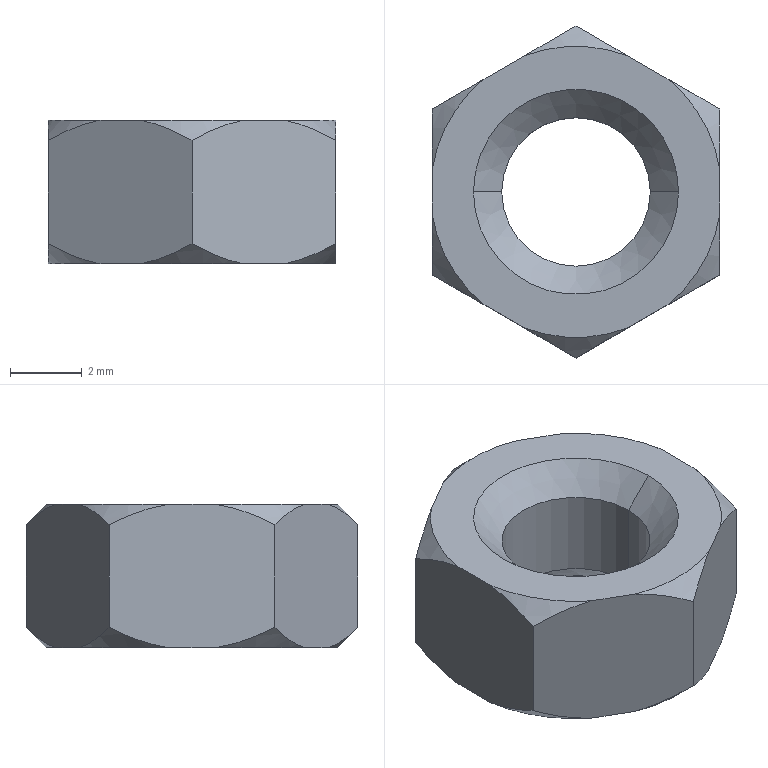Part | NX | features BREP 1 | 1 solid | 26 faces | box 8 x 9.238 x 4 mm | volume 157.518 mm3 | cone 16 | plane 8 | cylinder 2 | commonest cylinder face diameters 4.134 x2
STEP:
#1=CARTESIAN_POINT('',(-2.067,0.,-3.213));
#2=VERTEX_POINT('',#1);
#3=CARTESIAN_POINT('',(2.067,0.,-3.213));
#4=VERTEX_POINT('',#3);
#5=CARTESIAN_POINT('',(0.,0.,-3.213));
#6=DIRECTION('',(0.,0.,1.));
#7=DIRECTION('',(1.,0.,0.));
#8=AXIS2_PLACEMENT_3D('',#5,#6,#7);
#9=CIRCLE('',#8,2.067);
#10=EDGE_CURVE('',#2,#4,#9,.T.);
#11=ORIENTED_EDGE('',*,*,#10,.T.);
#12=CARTESIAN_POINT('',(2.854,0.,-4.));
#13=VERTEX_POINT('',#12);
#14=CARTESIAN_POINT('',(2.067,0.,-3.213));
#15=DIRECTION('',(0.7071,0.,-0.7071));
#16=VECTOR('',#15,1000.);
#17=LINE('',#14,#16);
#18=EDGE_CURVE('',#13,#4,#17,.F.);
#19=ORIENTED_EDGE('',*,*,#18,.F.);
#20=CARTESIAN_POINT('',(-2.854,0.,-4.));
#21=VERTEX_POINT('',#20);
#22=CARTESIAN_POINT('',(0.,0.,-4.));
#23=DIRECTION('',(0.,0.,1.));
#24=DIRECTION('',(1.,0.,0.));
#25=AXIS2_PLACEMENT_3D('',#22,#23,#24);
#26=CIRCLE('',#25,2.854);
#27=EDGE_CURVE('',#21,#13,#26,.T.);
#28=ORIENTED_EDGE('',*,*,#27,.F.);
#29=CARTESIAN_POINT('',(-2.067,0.,-3.213));
#30=DIRECTION('',(-0.7071,0.,-0.7071));
#31=VECTOR('',#30,1000.);
#32=LINE('',#29,#31);
#33=EDGE_CURVE('',#21,#2,#32,.F.);
#34=ORIENTED_EDGE('',*,*,#33,.T.);
#35=EDGE_LOOP('',(#11,#19,#28,#34));
#36=FACE_BOUND('',#35,.T.);
#37=CARTESIAN_POINT('',(0.,0.,-3.213));
#38=DIRECTION('',(0.,0.,-1.));
#39=DIRECTION('',(1.,0.,0.));
#40=AXIS2_PLACEMENT_3D('',#37,#38,#39);
#41=CONICAL_SURFACE('',#40,2.067,0.7854);
#42=ADVANCED_FACE('',(#36),#41,.F.);
#43=ORIENTED_EDGE('',*,*,#10,.F.);
#44=CARTESIAN_POINT('',(-2.067,0.,-0.7866));
#45=VERTEX_POINT('',#44);
#46=CARTESIAN_POINT('',(-2.067,0.,-23.));
#47=DIRECTION('',(0.,0.,1.));
#48=VECTOR('',#47,1000.);
#49=LINE('',#46,#48);
#50=EDGE_CURVE('',#2,#45,#49,.T.);
#51=ORIENTED_EDGE('',*,*,#50,.T.);
#52=CARTESIAN_POINT('',(2.067,0.,-0.7866));
#53=VERTEX_POINT('',#52);
#54=CARTESIAN_POINT('',(0.,0.,-0.7866));
#55=DIRECTION('',(0.,0.,1.));
#56=DIRECTION('',(1.,0.,0.));
#57=AXIS2_PLACEMENT_3D('',#54,#55,#56);
#58=CIRCLE('',#57,2.067);
#59=EDGE_CURVE('',#45,#53,#58,.T.);
#60=ORIENTED_EDGE('',*,*,#59,.T.);
#61=CARTESIAN_POINT('',(2.067,0.,-23.));
#62=DIRECTION('',(0.,0.,1.));
#63=VECTOR('',#62,1000.);
#64=LINE('',#61,#63);
#65=EDGE_CURVE('',#4,#53,#64,.T.);
#66=ORIENTED_EDGE('',*,*,#65,.F.);
#67=EDGE_LOOP('',(#43,#51,#60,#66));
#68=FACE_BOUND('',#67,.T.);
#69=CARTESIAN_POINT('',(0.,0.,-23.));
#70=DIRECTION('',(0.,0.,1.));
#71=DIRECTION('',(-1.,0.,0.));
#72=AXIS2_PLACEMENT_3D('',#69,#70,#71);
#73=CYLINDRICAL_SURFACE('',#72,2.067);
#74=ADVANCED_FACE('',(#68),#73,.F.);
#75=ORIENTED_EDGE('',*,*,#59,.F.);
#76=CARTESIAN_POINT('',(-2.854,0.,0.));
#77=VERTEX_POINT('',#76);
#78=CARTESIAN_POINT('',(-2.854,0.,0.));
#79=DIRECTION('',(-0.7071,0.,0.7071));
#80=VECTOR('',#79,1000.);
#81=LINE('',#78,#80);
#82=EDGE_CURVE('',#45,#77,#81,.T.);
#83=ORIENTED_EDGE('',*,*,#82,.T.);
#84=CARTESIAN_POINT('',(2.854,0.,0.));
#85=VERTEX_POINT('',#84);
#86=CARTESIAN_POINT('',(0.,0.,0.));
#87=DIRECTION('',(0.,0.,1.));
#88=DIRECTION('',(1.,0.,0.));
#89=AXIS2_PLACEMENT_3D('',#86,#87,#88);
#90=CIRCLE('',#89,2.854);
#91=EDGE_CURVE('',#77,#85,#90,.T.);
#92=ORIENTED_EDGE('',*,*,#91,.T.);
#93=CARTESIAN_POINT('',(2.854,0.,0.));
#94=DIRECTION('',(0.7071,0.,0.7071));
#95=VECTOR('',#94,1000.);
#96=LINE('',#93,#95);
#97=EDGE_CURVE('',#53,#85,#96,.T.);
#98=ORIENTED_EDGE('',*,*,#97,.F.);
#99=EDGE_LOOP('',(#75,#83,#92,#98));
#100=FACE_BOUND('',#99,.T.);
#101=CARTESIAN_POINT('',(0.,0.,0.));
#102=DIRECTION('',(0.,0.,1.));
#103=DIRECTION('',(-1.,0.,0.));
#104=AXIS2_PLACEMENT_3D('',#101,#102,#103);
#105=CONICAL_SURFACE('',#104,2.854,0.7854);
#106=ADVANCED_FACE('',(#100),#105,.F.);
#107=CARTESIAN_POINT('',(-4.,0.6483,0.));
#108=VERTEX_POINT('',#107);
#109=CARTESIAN_POINT('',(-4.,2.309,-0.5666));
#110=VERTEX_POINT('',#109);
#111=CARTESIAN_POINT('',(-4.,0.6483,0.));
#112=CARTESIAN_POINT('',(-4.,1.234,-0.09377));
#113=CARTESIAN_POINT('',(-4.,1.781,-0.3026));
#114=CARTESIAN_POINT('',(-4.,2.309,-0.5666));
#115=B_SPLINE_CURVE_WITH_KNOTS('',3,(#111,#112,#113,#114),.UNSPECIFIED.,.F.,.F.,(4,4),(0.,0.001755),.UNSPECIFIED.);
#116=EDGE_CURVE('',#108,#110,#115,.T.);
#117=ORIENTED_EDGE('',*,*,#116,.F.);
#118=CARTESIAN_POINT('',(-2.561,3.14,0.));
#119=VERTEX_POINT('',#118);
#120=CARTESIAN_POINT('',(0.,0.,0.));
#121=DIRECTION('',(0.,0.,1.));
#122=DIRECTION('',(1.,0.,0.));
#123=AXIS2_PLACEMENT_3D('',#120,#121,#122);
#124=CIRCLE('',#123,4.052);
#125=EDGE_CURVE('',#119,#108,#124,.T.);
#126=ORIENTED_EDGE('',*,*,#125,.F.);
#127=CARTESIAN_POINT('',(-4.,2.309,-0.5666));
#128=CARTESIAN_POINT('',(-3.543,2.573,-0.3026));
#129=CARTESIAN_POINT('',(-3.069,2.847,-0.09377));
#130=CARTESIAN_POINT('',(-2.561,3.14,0.));
#131=B_SPLINE_CURVE_WITH_KNOTS('',3,(#127,#128,#129,#130),.UNSPECIFIED.,.F.,.F.,(4,4),(0.,0.001755),.UNSPECIFIED.);
#132=EDGE_CURVE('',#110,#119,#131,.T.);
#133=ORIENTED_EDGE('',*,*,#132,.F.);
#134=EDGE_LOOP('',(#117,#126,#133));
#135=FACE_BOUND('',#134,.T.);
#136=CARTESIAN_POINT('',(0.,0.,-0.9428));
#137=DIRECTION('',(0.,0.,-1.));
#138=DIRECTION('',(1.,0.,0.));
#139=AXIS2_PLACEMENT_3D('',#136,#137,#138);
#140=CONICAL_SURFACE('',#139,4.995,0.7854);
#141=ADVANCED_FACE('',(#135),#140,.T.);
#142=CARTESIAN_POINT('',(-1.439,3.788,0.));
#143=VERTEX_POINT('',#142);
#144=CARTESIAN_POINT('',(0.,4.619,-0.5666));
#145=VERTEX_POINT('',#144);
#146=CARTESIAN_POINT('',(-1.439,3.788,0.));
#147=CARTESIAN_POINT('',(-1.187,3.933,-0.04639));
#148=CARTESIAN_POINT('',(-0.9421,4.075,-0.122));
#149=CARTESIAN_POINT('',(-0.4604,4.353,-0.3173));
#150=CARTESIAN_POINT('',(-0.2261,4.488,-0.4361));
#151=CARTESIAN_POINT('',(0.,4.619,-0.5666));
#152=B_SPLINE_CURVE_WITH_KNOTS('',3,(#146,#147,#148,#149,#150,#151),.UNSPECIFIED.,.F.,.F.,(4,2,4),(0.,0.5,1.),.UNSPECIFIED.);
#153=EDGE_CURVE('',#143,#145,#152,.T.);
#154=ORIENTED_EDGE('',*,*,#153,.F.);
#155=CARTESIAN_POINT('',(1.439,3.788,0.));
#156=VERTEX_POINT('',#155);
#157=CARTESIAN_POINT('',(0.,0.,0.));
#158=DIRECTION('',(0.,0.,1.));
#159=DIRECTION('',(1.,0.,0.));
#160=AXIS2_PLACEMENT_3D('',#157,#158,#159);
#161=CIRCLE('',#160,4.052);
#162=EDGE_CURVE('',#156,#143,#161,.T.);
#163=ORIENTED_EDGE('',*,*,#162,.F.);
#164=CARTESIAN_POINT('',(0.,4.619,-0.5666));
#165=CARTESIAN_POINT('',(0.4573,4.355,-0.3026));
#166=CARTESIAN_POINT('',(0.931,4.081,-0.09377));
#167=CARTESIAN_POINT('',(1.439,3.788,0.));
#168=B_SPLINE_CURVE_WITH_KNOTS('',3,(#164,#165,#166,#167),.UNSPECIFIED.,.F.,.F.,(4,4),(0.,0.001755),.UNSPECIFIED.);
#169=EDGE_CURVE('',#145,#156,#168,.T.);
#170=ORIENTED_EDGE('',*,*,#169,.F.);
#171=EDGE_LOOP('',(#154,#163,#170));
#172=FACE_BOUND('',#171,.T.);
#173=CARTESIAN_POINT('',(0.,0.,-0.9428));
#174=DIRECTION('',(0.,0.,-1.));
#175=DIRECTION('',(1.,0.,0.));
#176=AXIS2_PLACEMENT_3D('',#173,#174,#175);
#177=CONICAL_SURFACE('',#176,4.995,0.7854);
#178=ADVANCED_FACE('',(#172),#177,.T.);
#179=CARTESIAN_POINT('',(2.561,3.14,0.));
#180=VERTEX_POINT('',#179);
#181=CARTESIAN_POINT('',(4.,2.309,-0.5666));
#182=VERTEX_POINT('',#181);
#183=CARTESIAN_POINT('',(2.561,3.14,0.));
#184=CARTESIAN_POINT('',(2.813,2.995,-0.04639));
#185=CARTESIAN_POINT('',(3.058,2.853,-0.122));
#186=CARTESIAN_POINT('',(3.54,2.575,-0.3173));
#187=CARTESIAN_POINT('',(3.774,2.44,-0.4361));
#188=CARTESIAN_POINT('',(4.,2.309,-0.5666));
#189=B_SPLINE_CURVE_WITH_KNOTS('',3,(#183,#184,#185,#186,#187,#188),.UNSPECIFIED.,.F.,.F.,(4,2,4),(0.,0.5,1.),.UNSPECIFIED.);
#190=EDGE_CURVE('',#180,#182,#189,.T.);
#191=ORIENTED_EDGE('',*,*,#190,.F.);
#192=CARTESIAN_POINT('',(4.,0.6483,0.));
#193=VERTEX_POINT('',#192);
#194=CARTESIAN_POINT('',(0.,0.,0.));
#195=DIRECTION('',(0.,0.,1.));
#196=DIRECTION('',(1.,0.,0.));
#197=AXIS2_PLACEMENT_3D('',#194,#195,#196);
#198=CIRCLE('',#197,4.052);
#199=EDGE_CURVE('',#193,#180,#198,.T.);
#200=ORIENTED_EDGE('',*,*,#199,.F.);
#201=CARTESIAN_POINT('',(4.,2.309,-0.5666));
#202=CARTESIAN_POINT('',(4.,1.781,-0.3026));
#203=CARTESIAN_POINT('',(4.,1.234,-0.09377));
#204=CARTESIAN_POINT('',(4.,0.6483,0.));
#205=B_SPLINE_CURVE_WITH_KNOTS('',3,(#201,#202,#203,#204),.UNSPECIFIED.,.F.,.F.,(4,4),(0.,0.001755),.UNSPECIFIED.);
#206=EDGE_CURVE('',#182,#193,#205,.T.);
#207=ORIENTED_EDGE('',*,*,#206,.F.);
#208=EDGE_LOOP('',(#191,#200,#207));
#209=FACE_BOUND('',#208,.T.);
#210=CARTESIAN_POINT('',(0.,0.,-0.9428));
#211=DIRECTION('',(0.,0.,-1.));
#212=DIRECTION('',(1.,0.,0.));
#213=AXIS2_PLACEMENT_3D('',#210,#211,#212);
#214=CONICAL_SURFACE('',#213,4.995,0.7854);
#215=ADVANCED_FACE('',(#209),#214,.T.);
#216=CARTESIAN_POINT('',(4.,-0.6483,0.));
#217=VERTEX_POINT('',#216);
#218=CARTESIAN_POINT('',(4.,-2.309,-0.5666));
#219=VERTEX_POINT('',#218);
#220=CARTESIAN_POINT('',(4.,-0.6483,0.));
#221=CARTESIAN_POINT('',(4.,-1.234,-0.09377));
#222=CARTESIAN_POINT('',(4.,-1.781,-0.3026));
#223=CARTESIAN_POINT('',(4.,-2.309,-0.5666));
#224=B_SPLINE_CURVE_WITH_KNOTS('',3,(#220,#221,#222,#223),.UNSPECIFIED.,.F.,.F.,(4,4),(0.,0.001755),.UNSPECIFIED.);
#225=EDGE_CURVE('',#217,#219,#224,.T.);
#226=ORIENTED_EDGE('',*,*,#225,.F.);
#227=CARTESIAN_POINT('',(2.561,-3.14,0.));
#228=VERTEX_POINT('',#227);
#229=CARTESIAN_POINT('',(0.,0.,0.));
#230=DIRECTION('',(0.,0.,1.));
#231=DIRECTION('',(1.,0.,0.));
#232=AXIS2_PLACEMENT_3D('',#229,#230,#231);
#233=CIRCLE('',#232,4.052);
#234=EDGE_CURVE('',#228,#217,#233,.T.);
#235=ORIENTED_EDGE('',*,*,#234,.F.);
#236=CARTESIAN_POINT('',(4.,-2.309,-0.5666));
#237=CARTESIAN_POINT('',(3.543,-2.573,-0.3026));
#238=CARTESIAN_POINT('',(3.069,-2.847,-0.09377));
#239=CARTESIAN_POINT('',(2.561,-3.14,0.));
#240=B_SPLINE_CURVE_WITH_KNOTS('',3,(#236,#237,#238,#239),.UNSPECIFIED.,.F.,.F.,(4,4),(0.,0.001755),.UNSPECIFIED.);
#241=EDGE_CURVE('',#219,#228,#240,.T.);
#242=ORIENTED_EDGE('',*,*,#241,.F.);
#243=EDGE_LOOP('',(#226,#235,#242));
#244=FACE_BOUND('',#243,.T.);
#245=CARTESIAN_POINT('',(0.,0.,-0.9428));
#246=DIRECTION('',(0.,0.,-1.));
#247=DIRECTION('',(1.,0.,0.));
#248=AXIS2_PLACEMENT_3D('',#245,#246,#247);
#249=CONICAL_SURFACE('',#248,4.995,0.7854);
#250=ADVANCED_FACE('',(#244),#249,.T.);
#251=CARTESIAN_POINT('',(1.439,-3.788,0.));
#252=VERTEX_POINT('',#251);
#253=CARTESIAN_POINT('',(0.,-4.619,-0.5666));
#254=VERTEX_POINT('',#253);
#255=CARTESIAN_POINT('',(1.439,-3.788,0.));
#256=CARTESIAN_POINT('',(1.187,-3.933,-0.04639));
#257=CARTESIAN_POINT('',(0.9421,-4.075,-0.122));
#258=CARTESIAN_POINT('',(0.4604,-4.353,-0.3173));
#259=CARTESIAN_POINT('',(0.2261,-4.488,-0.4361));
#260=CARTESIAN_POINT('',(0.,-4.619,-0.5666));
#261=B_SPLINE_CURVE_WITH_KNOTS('',3,(#255,#256,#257,#258,#259,#260),.UNSPECIFIED.,.F.,.F.,(4,2,4),(0.,0.5,1.),.UNSPECIFIED.);
#262=EDGE_CURVE('',#252,#254,#261,.T.);
#263=ORIENTED_EDGE('',*,*,#262,.F.);
#264=CARTESIAN_POINT('',(-1.439,-3.788,0.));
#265=VERTEX_POINT('',#264);
#266=CARTESIAN_POINT('',(0.,0.,0.));
#267=DIRECTION('',(0.,0.,1.));
#268=DIRECTION('',(1.,0.,0.));
#269=AXIS2_PLACEMENT_3D('',#266,#267,#268);
#270=CIRCLE('',#269,4.052);
#271=EDGE_CURVE('',#265,#252,#270,.T.);
#272=ORIENTED_EDGE('',*,*,#271,.F.);
#273=CARTESIAN_POINT('',(0.,-4.619,-0.5666));
#274=CARTESIAN_POINT('',(-0.4573,-4.355,-0.3026));
#275=CARTESIAN_POINT('',(-0.931,-4.081,-0.09377));
#276=CARTESIAN_POINT('',(-1.439,-3.788,0.));
#277=B_SPLINE_CURVE_WITH_KNOTS('',3,(#273,#274,#275,#276),.UNSPECIFIED.,.F.,.F.,(4,4),(0.,0.001755),.UNSPECIFIED.);
#278=EDGE_CURVE('',#254,#265,#277,.T.);
#279=ORIENTED_EDGE('',*,*,#278,.F.);
#280=EDGE_LOOP('',(#263,#272,#279));
#281=FACE_BOUND('',#280,.T.);
#282=CARTESIAN_POINT('',(0.,0.,-0.9428));
#283=DIRECTION('',(0.,0.,-1.));
#284=DIRECTION('',(1.,0.,0.));
#285=AXIS2_PLACEMENT_3D('',#282,#283,#284);
#286=CONICAL_SURFACE('',#285,4.995,0.7854);
#287=ADVANCED_FACE('',(#281),#286,.T.);
#288=CARTESIAN_POINT('',(-4.,-2.309,-0.5666));
#289=VERTEX_POINT('',#288);
#290=CARTESIAN_POINT('',(-4.,-0.6483,0.));
#291=VERTEX_POINT('',#290);
#292=CARTESIAN_POINT('',(-4.,-2.309,-0.5666));
#293=CARTESIAN_POINT('',(-4.,-1.781,-0.3026));
#294=CARTESIAN_POINT('',(-4.,-1.234,-0.09377));
#295=CARTESIAN_POINT('',(-4.,-0.6483,0.));
#296=B_SPLINE_CURVE_WITH_KNOTS('',3,(#292,#293,#294,#295),.UNSPECIFIED.,.F.,.F.,(4,4),(0.,0.001755),.UNSPECIFIED.);
#297=EDGE_CURVE('',#289,#291,#296,.T.);
#298=ORIENTED_EDGE('',*,*,#297,.F.);
#299=CARTESIAN_POINT('',(-2.561,-3.14,0.));
#300=VERTEX_POINT('',#299);
#301=CARTESIAN_POINT('',(-2.561,-3.14,0.));
#302=CARTESIAN_POINT('',(-2.813,-2.995,-0.04639));
#303=CARTESIAN_POINT('',(-3.058,-2.853,-0.122));
#304=CARTESIAN_POINT('',(-3.54,-2.575,-0.3173));
#305=CARTESIAN_POINT('',(-3.774,-2.44,-0.4361));
#306=CARTESIAN_POINT('',(-4.,-2.309,-0.5666));
#307=B_SPLINE_CURVE_WITH_KNOTS('',3,(#301,#302,#303,#304,#305,#306),.UNSPECIFIED.,.F.,.F.,(4,2,4),(0.,0.5,1.),.UNSPECIFIED.);
#308=EDGE_CURVE('',#300,#289,#307,.T.);
#309=ORIENTED_EDGE('',*,*,#308,.F.);
#310=CARTESIAN_POINT('',(0.,0.,0.));
#311=DIRECTION('',(0.,0.,1.));
#312=DIRECTION('',(1.,0.,0.));
#313=AXIS2_PLACEMENT_3D('',#310,#311,#312);
#314=CIRCLE('',#313,4.052);
#315=EDGE_CURVE('',#291,#300,#314,.T.);
#316=ORIENTED_EDGE('',*,*,#315,.F.);
#317=EDGE_LOOP('',(#298,#309,#316));
#318=FACE_BOUND('',#317,.T.);
#319=CARTESIAN_POINT('',(0.,0.,-0.9428));
#320=DIRECTION('',(0.,0.,-1.));
#321=DIRECTION('',(1.,0.,0.));
#322=AXIS2_PLACEMENT_3D('',#319,#320,#321);
#323=CONICAL_SURFACE('',#322,4.995,0.7854);
#324=ADVANCED_FACE('',(#318),#323,.T.);
#325=CARTESIAN_POINT('',(0.,0.,0.));
#326=DIRECTION('',(0.,0.,1.));
#327=DIRECTION('',(1.,0.,0.));
#328=AXIS2_PLACEMENT_3D('',#325,#326,#327);
#329=CIRCLE('',#328,2.854);
#330=EDGE_CURVE('',#85,#77,#329,.T.);
#331=ORIENTED_EDGE('',*,*,#330,.F.);
#332=ORIENTED_EDGE('',*,*,#91,.F.);
#333=EDGE_LOOP('',(#331,#332));
#334=FACE_BOUND('',#333,.T.);
#335=CARTESIAN_POINT('',(-4.,2.309,0.));
#336=DIRECTION('',(0.,-1.,0.));
#337=VECTOR('',#336,1000.);
#338=LINE('',#335,#337);
#339=EDGE_CURVE('',#108,#291,#338,.T.);
#340=ORIENTED_EDGE('',*,*,#339,.T.);
#341=ORIENTED_EDGE('',*,*,#315,.T.);
#342=CARTESIAN_POINT('',(-4.,-2.309,0.));
#343=DIRECTION('',(0.866,-0.5,0.));
#344=VECTOR('',#343,1000.);
#345=LINE('',#342,#344);
#346=EDGE_CURVE('',#300,#265,#345,.T.);
#347=ORIENTED_EDGE('',*,*,#346,.T.);
#348=ORIENTED_EDGE('',*,*,#271,.T.);
#349=CARTESIAN_POINT('',(0.,-4.619,0.));
#350=DIRECTION('',(0.866,0.5,0.));
#351=VECTOR('',#350,1000.);
#352=LINE('',#349,#351);
#353=EDGE_CURVE('',#252,#228,#352,.T.);
#354=ORIENTED_EDGE('',*,*,#353,.T.);
#355=ORIENTED_EDGE('',*,*,#234,.T.);
#356=CARTESIAN_POINT('',(4.,-2.309,0.));
#357=DIRECTION('',(0.,1.,0.));
#358=VECTOR('',#357,1000.);
#359=LINE('',#356,#358);
#360=EDGE_CURVE('',#217,#193,#359,.T.);
#361=ORIENTED_EDGE('',*,*,#360,.T.);
#362=ORIENTED_EDGE('',*,*,#199,.T.);
#363=CARTESIAN_POINT('',(4.,2.309,0.));
#364=DIRECTION('',(-0.866,0.5,0.));
#365=VECTOR('',#364,1000.);
#366=LINE('',#363,#365);
#367=EDGE_CURVE('',#180,#156,#366,.T.);
#368=ORIENTED_EDGE('',*,*,#367,.T.);
#369=ORIENTED_EDGE('',*,*,#162,.T.);
#370=CARTESIAN_POINT('',(0.,4.619,0.));
#371=DIRECTION('',(-0.866,-0.5,0.));
#372=VECTOR('',#371,1000.);
#373=LINE('',#370,#372);
#374=EDGE_CURVE('',#143,#119,#373,.T.);
#375=ORIENTED_EDGE('',*,*,#374,.T.);
#376=ORIENTED_EDGE('',*,*,#125,.T.);
#377=EDGE_LOOP('',(#340,#341,#347,#348,#354,#355,#361,#362,#368,#369,#375,#376));
#378=FACE_BOUND('',#377,.T.);
#379=CARTESIAN_POINT('',(0.,4.052,0.));
#380=DIRECTION('',(0.,0.,-1.));
#381=DIRECTION('',(1.,0.,0.));
#382=AXIS2_PLACEMENT_3D('',#379,#380,#381);
#383=PLANE('',#382);
#384=ADVANCED_FACE('',(#334,#378),#383,.F.);
#385=ORIENTED_EDGE('',*,*,#27,.T.);
#386=CARTESIAN_POINT('',(0.,0.,-4.));
#387=DIRECTION('',(0.,0.,1.));
#388=DIRECTION('',(1.,0.,0.));
#389=AXIS2_PLACEMENT_3D('',#386,#387,#388);
#390=CIRCLE('',#389,2.854);
#391=EDGE_CURVE('',#13,#21,#390,.T.);
#392=ORIENTED_EDGE('',*,*,#391,.T.);
#393=EDGE_LOOP('',(#385,#392));
#394=FACE_BOUND('',#393,.T.);
#395=CARTESIAN_POINT('',(-4.,0.6483,-4.));
#396=VERTEX_POINT('',#395);
#397=CARTESIAN_POINT('',(-4.,-0.6483,-4.));
#398=VERTEX_POINT('',#397);
#399=CARTESIAN_POINT('',(-4.,2.854,-4.));
#400=DIRECTION('',(0.,-1.,0.));
#401=VECTOR('',#400,1000.);
#402=LINE('',#399,#401);
#403=EDGE_CURVE('',#396,#398,#402,.T.);
#404=ORIENTED_EDGE('',*,*,#403,.F.);
#405=CARTESIAN_POINT('',(-2.561,3.14,-4.));
#406=VERTEX_POINT('',#405);
#407=CARTESIAN_POINT('',(0.,0.,-4.));
#408=DIRECTION('',(0.,0.,1.));
#409=DIRECTION('',(1.,0.,0.));
#410=AXIS2_PLACEMENT_3D('',#407,#408,#409);
#411=CIRCLE('',#410,4.052);
#412=EDGE_CURVE('',#406,#396,#411,.T.);
#413=ORIENTED_EDGE('',*,*,#412,.F.);
#414=CARTESIAN_POINT('',(-1.439,3.788,-4.));
#415=VERTEX_POINT('',#414);
#416=CARTESIAN_POINT('',(-0.7644,4.177,-4.));
#417=DIRECTION('',(-0.866,-0.5,0.));
#418=VECTOR('',#417,1000.);
#419=LINE('',#416,#418);
#420=EDGE_CURVE('',#415,#406,#419,.T.);
#421=ORIENTED_EDGE('',*,*,#420,.F.);
#422=CARTESIAN_POINT('',(1.439,3.788,-4.));
#423=VERTEX_POINT('',#422);
#424=CARTESIAN_POINT('',(0.,0.,-4.));
#425=DIRECTION('',(0.,0.,1.));
#426=DIRECTION('',(1.,0.,0.));
#427=AXIS2_PLACEMENT_3D('',#424,#425,#426);
#428=CIRCLE('',#427,4.052);
#429=EDGE_CURVE('',#423,#415,#428,.T.);
#430=ORIENTED_EDGE('',*,*,#429,.F.);
#431=CARTESIAN_POINT('',(2.561,3.14,-4.));
#432=VERTEX_POINT('',#431);
#433=CARTESIAN_POINT('',(0.7644,4.177,-4.));
#434=DIRECTION('',(-0.866,0.5,0.));
#435=VECTOR('',#434,1000.);
#436=LINE('',#433,#435);
#437=EDGE_CURVE('',#432,#423,#436,.T.);
#438=ORIENTED_EDGE('',*,*,#437,.F.);
#439=CARTESIAN_POINT('',(4.,0.6483,-4.));
#440=VERTEX_POINT('',#439);
#441=CARTESIAN_POINT('',(0.,0.,-4.));
#442=DIRECTION('',(0.,0.,1.));
#443=DIRECTION('',(1.,0.,0.));
#444=AXIS2_PLACEMENT_3D('',#441,#442,#443);
#445=CIRCLE('',#444,4.052);
#446=EDGE_CURVE('',#440,#432,#445,.T.);
#447=ORIENTED_EDGE('',*,*,#446,.F.);
#448=CARTESIAN_POINT('',(4.,-0.6483,-4.));
#449=VERTEX_POINT('',#448);
#450=CARTESIAN_POINT('',(4.,2.854,-4.));
#451=DIRECTION('',(0.,1.,0.));
#452=VECTOR('',#451,1000.);
#453=LINE('',#450,#452);
#454=EDGE_CURVE('',#449,#440,#453,.T.);
#455=ORIENTED_EDGE('',*,*,#454,.F.);
#456=CARTESIAN_POINT('',(2.561,-3.14,-4.));
#457=VERTEX_POINT('',#456);
#458=CARTESIAN_POINT('',(0.,0.,-4.));
#459=DIRECTION('',(0.,0.,1.));
#460=DIRECTION('',(1.,0.,0.));
#461=AXIS2_PLACEMENT_3D('',#458,#459,#460);
#462=CIRCLE('',#461,4.052);
#463=EDGE_CURVE('',#457,#449,#462,.T.);
#464=ORIENTED_EDGE('',*,*,#463,.F.);
#465=CARTESIAN_POINT('',(1.439,-3.788,-4.));
#466=VERTEX_POINT('',#465);
#467=CARTESIAN_POINT('',(3.236,-2.751,-4.));
#468=DIRECTION('',(0.866,0.5,0.));
#469=VECTOR('',#468,1000.);
#470=LINE('',#467,#469);
#471=EDGE_CURVE('',#466,#457,#470,.T.);
#472=ORIENTED_EDGE('',*,*,#471,.F.);
#473=CARTESIAN_POINT('',(-1.439,-3.788,-4.));
#474=VERTEX_POINT('',#473);
#475=CARTESIAN_POINT('',(0.,0.,-4.));
#476=DIRECTION('',(0.,0.,1.));
#477=DIRECTION('',(1.,0.,0.));
#478=AXIS2_PLACEMENT_3D('',#475,#476,#477);
#479=CIRCLE('',#478,4.052);
#480=EDGE_CURVE('',#474,#466,#479,.T.);
#481=ORIENTED_EDGE('',*,*,#480,.F.);
#482=CARTESIAN_POINT('',(-2.561,-3.14,-4.));
#483=VERTEX_POINT('',#482);
#484=CARTESIAN_POINT('',(-3.236,-2.751,-4.));
#485=DIRECTION('',(0.866,-0.5,0.));
#486=VECTOR('',#485,1000.);
#487=LINE('',#484,#486);
#488=EDGE_CURVE('',#483,#474,#487,.T.);
#489=ORIENTED_EDGE('',*,*,#488,.F.);
#490=CARTESIAN_POINT('',(0.,0.,-4.));
#491=DIRECTION('',(0.,0.,1.));
#492=DIRECTION('',(1.,0.,0.));
#493=AXIS2_PLACEMENT_3D('',#490,#491,#492);
#494=CIRCLE('',#493,4.052);
#495=EDGE_CURVE('',#398,#483,#494,.T.);
#496=ORIENTED_EDGE('',*,*,#495,.F.);
#497=EDGE_LOOP('',(#404,#413,#421,#430,#438,#447,#455,#464,#472,#481,#489,#496));
#498=FACE_BOUND('',#497,.T.);
#499=CARTESIAN_POINT('',(0.,2.854,-4.));
#500=DIRECTION('',(0.,0.,1.));
#501=DIRECTION('',(-1.,0.,0.));
#502=AXIS2_PLACEMENT_3D('',#499,#500,#501);
#503=PLANE('',#502);
#504=ADVANCED_FACE('',(#394,#498),#503,.F.);
#505=CARTESIAN_POINT('',(-4.,2.309,-3.433));
#506=VERTEX_POINT('',#505);
#507=CARTESIAN_POINT('',(-4.,2.309,-3.433));
#508=CARTESIAN_POINT('',(-4.,1.781,-3.697));
#509=CARTESIAN_POINT('',(-4.,1.234,-3.906));
#510=CARTESIAN_POINT('',(-4.,0.6483,-4.));
#511=B_SPLINE_CURVE_WITH_KNOTS('',3,(#507,#508,#509,#510),.UNSPECIFIED.,.F.,.F.,(4,4),(0.,0.001755),.UNSPECIFIED.);
#512=EDGE_CURVE('',#506,#396,#511,.T.);
#513=ORIENTED_EDGE('',*,*,#512,.F.);
#514=CARTESIAN_POINT('',(-2.561,3.14,-4.));
#515=CARTESIAN_POINT('',(-2.813,2.995,-3.954));
#516=CARTESIAN_POINT('',(-3.058,2.853,-3.878));
#517=CARTESIAN_POINT('',(-3.54,2.575,-3.683));
#518=CARTESIAN_POINT('',(-3.774,2.44,-3.564));
#519=CARTESIAN_POINT('',(-4.,2.309,-3.433));
#520=B_SPLINE_CURVE_WITH_KNOTS('',3,(#514,#515,#516,#517,#518,#519),.UNSPECIFIED.,.F.,.F.,(4,2,4),(0.,0.5,1.),.UNSPECIFIED.);
#521=EDGE_CURVE('',#406,#506,#520,.T.);
#522=ORIENTED_EDGE('',*,*,#521,.F.);
#523=ORIENTED_EDGE('',*,*,#412,.T.);
#524=EDGE_LOOP('',(#513,#522,#523));
#525=FACE_BOUND('',#524,.T.);
#526=CARTESIAN_POINT('',(0.,0.,-4.));
#527=DIRECTION('',(0.,0.,1.));
#528=DIRECTION('',(-1.,0.,0.));
#529=AXIS2_PLACEMENT_3D('',#526,#527,#528);
#530=CONICAL_SURFACE('',#529,4.052,0.7854);
#531=ADVANCED_FACE('',(#525),#530,.T.);
#532=CARTESIAN_POINT('',(0.,4.619,-3.433));
#533=VERTEX_POINT('',#532);
#534=CARTESIAN_POINT('',(0.,4.619,-3.433));
#535=CARTESIAN_POINT('',(-0.4573,4.355,-3.697));
#536=CARTESIAN_POINT('',(-0.931,4.081,-3.906));
#537=CARTESIAN_POINT('',(-1.439,3.788,-4.));
#538=B_SPLINE_CURVE_WITH_KNOTS('',3,(#534,#535,#536,#537),.UNSPECIFIED.,.F.,.F.,(4,4),(0.,0.001755),.UNSPECIFIED.);
#539=EDGE_CURVE('',#533,#415,#538,.T.);
#540=ORIENTED_EDGE('',*,*,#539,.F.);
#541=CARTESIAN_POINT('',(1.439,3.788,-4.));
#542=CARTESIAN_POINT('',(1.187,3.933,-3.954));
#543=CARTESIAN_POINT('',(0.9421,4.075,-3.878));
#544=CARTESIAN_POINT('',(0.4604,4.353,-3.683));
#545=CARTESIAN_POINT('',(0.2261,4.488,-3.564));
#546=CARTESIAN_POINT('',(0.,4.619,-3.433));
#547=B_SPLINE_CURVE_WITH_KNOTS('',3,(#541,#542,#543,#544,#545,#546),.UNSPECIFIED.,.F.,.F.,(4,2,4),(0.,0.5,1.),.UNSPECIFIED.);
#548=EDGE_CURVE('',#423,#533,#547,.T.);
#549=ORIENTED_EDGE('',*,*,#548,.F.);
#550=ORIENTED_EDGE('',*,*,#429,.T.);
#551=EDGE_LOOP('',(#540,#549,#550));
#552=FACE_BOUND('',#551,.T.);
#553=CARTESIAN_POINT('',(0.,0.,-4.));
#554=DIRECTION('',(0.,0.,1.));
#555=DIRECTION('',(-1.,0.,0.));
#556=AXIS2_PLACEMENT_3D('',#553,#554,#555);
#557=CONICAL_SURFACE('',#556,4.052,0.7854);
#558=ADVANCED_FACE('',(#552),#557,.T.);
#559=CARTESIAN_POINT('',(4.,2.309,-3.433));
#560=VERTEX_POINT('',#559);
#561=CARTESIAN_POINT('',(4.,2.309,-3.433));
#562=CARTESIAN_POINT('',(3.543,2.573,-3.697));
#563=CARTESIAN_POINT('',(3.069,2.847,-3.906));
#564=CARTESIAN_POINT('',(2.561,3.14,-4.));
#565=B_SPLINE_CURVE_WITH_KNOTS('',3,(#561,#562,#563,#564),.UNSPECIFIED.,.F.,.F.,(4,4),(0.,0.001755),.UNSPECIFIED.);
#566=EDGE_CURVE('',#560,#432,#565,.T.);
#567=ORIENTED_EDGE('',*,*,#566,.F.);
#568=CARTESIAN_POINT('',(4.,0.6483,-4.));
#569=CARTESIAN_POINT('',(4.,1.234,-3.906));
#570=CARTESIAN_POINT('',(4.,1.781,-3.697));
#571=CARTESIAN_POINT('',(4.,2.309,-3.433));
#572=B_SPLINE_CURVE_WITH_KNOTS('',3,(#568,#569,#570,#571),.UNSPECIFIED.,.F.,.F.,(4,4),(0.,0.001755),.UNSPECIFIED.);
#573=EDGE_CURVE('',#440,#560,#572,.T.);
#574=ORIENTED_EDGE('',*,*,#573,.F.);
#575=ORIENTED_EDGE('',*,*,#446,.T.);
#576=EDGE_LOOP('',(#567,#574,#575));
#577=FACE_BOUND('',#576,.T.);
#578=CARTESIAN_POINT('',(0.,0.,-4.));
#579=DIRECTION('',(0.,0.,1.));
#580=DIRECTION('',(-1.,0.,0.));
#581=AXIS2_PLACEMENT_3D('',#578,#579,#580);
#582=CONICAL_SURFACE('',#581,4.052,0.7854);
#583=ADVANCED_FACE('',(#577),#582,.T.);
#584=CARTESIAN_POINT('',(4.,-2.309,-3.433));
#585=VERTEX_POINT('',#584);
#586=CARTESIAN_POINT('',(4.,-2.309,-3.433));
#587=CARTESIAN_POINT('',(4.,-1.781,-3.697));
#588=CARTESIAN_POINT('',(4.,-1.234,-3.906));
#589=CARTESIAN_POINT('',(4.,-0.6483,-4.));
#590=B_SPLINE_CURVE_WITH_KNOTS('',3,(#586,#587,#588,#589),.UNSPECIFIED.,.F.,.F.,(4,4),(0.,0.001755),.UNSPECIFIED.);
#591=EDGE_CURVE('',#585,#449,#590,.T.);
#592=ORIENTED_EDGE('',*,*,#591,.F.);
#593=CARTESIAN_POINT('',(2.561,-3.14,-4.));
#594=CARTESIAN_POINT('',(2.813,-2.995,-3.954));
#595=CARTESIAN_POINT('',(3.058,-2.853,-3.878));
#596=CARTESIAN_POINT('',(3.54,-2.575,-3.683));
#597=CARTESIAN_POINT('',(3.774,-2.44,-3.564));
#598=CARTESIAN_POINT('',(4.,-2.309,-3.433));
#599=B_SPLINE_CURVE_WITH_KNOTS('',3,(#593,#594,#595,#596,#597,#598),.UNSPECIFIED.,.F.,.F.,(4,2,4),(0.,0.5,1.),.UNSPECIFIED.);
#600=EDGE_CURVE('',#457,#585,#599,.T.);
#601=ORIENTED_EDGE('',*,*,#600,.F.);
#602=ORIENTED_EDGE('',*,*,#463,.T.);
#603=EDGE_LOOP('',(#592,#601,#602));
#604=FACE_BOUND('',#603,.T.);
#605=CARTESIAN_POINT('',(0.,0.,-4.));
#606=DIRECTION('',(0.,0.,1.));
#607=DIRECTION('',(-1.,0.,0.));
#608=AXIS2_PLACEMENT_3D('',#605,#606,#607);
#609=CONICAL_SURFACE('',#608,4.052,0.7854);
#610=ADVANCED_FACE('',(#604),#609,.T.);
#611=CARTESIAN_POINT('',(-4.,-2.309,-3.433));
#612=VERTEX_POINT('',#611);
#613=CARTESIAN_POINT('',(-4.,-0.6483,-4.));
#614=CARTESIAN_POINT('',(-4.,-1.234,-3.906));
#615=CARTESIAN_POINT('',(-4.,-1.781,-3.697));
#616=CARTESIAN_POINT('',(-4.,-2.309,-3.433));
#617=B_SPLINE_CURVE_WITH_KNOTS('',3,(#613,#614,#615,#616),.UNSPECIFIED.,.F.,.F.,(4,4),(0.,0.001755),.UNSPECIFIED.);
#618=EDGE_CURVE('',#398,#612,#617,.T.);
#619=ORIENTED_EDGE('',*,*,#618,.F.);
#620=ORIENTED_EDGE('',*,*,#495,.T.);
#621=CARTESIAN_POINT('',(-4.,-2.309,-3.433));
#622=CARTESIAN_POINT('',(-3.543,-2.573,-3.697));
#623=CARTESIAN_POINT('',(-3.069,-2.847,-3.906));
#624=CARTESIAN_POINT('',(-2.561,-3.14,-4.));
#625=B_SPLINE_CURVE_WITH_KNOTS('',3,(#621,#622,#623,#624),.UNSPECIFIED.,.F.,.F.,(4,4),(0.,0.001755),.UNSPECIFIED.);
#626=EDGE_CURVE('',#612,#483,#625,.T.);
#627=ORIENTED_EDGE('',*,*,#626,.F.);
#628=EDGE_LOOP('',(#619,#620,#627));
#629=FACE_BOUND('',#628,.T.);
#630=CARTESIAN_POINT('',(0.,0.,-4.));
#631=DIRECTION('',(0.,0.,1.));
#632=DIRECTION('',(-1.,0.,0.));
#633=AXIS2_PLACEMENT_3D('',#630,#631,#632);
#634=CONICAL_SURFACE('',#633,4.052,0.7854);
#635=ADVANCED_FACE('',(#629),#634,.T.);
#636=CARTESIAN_POINT('',(0.,-4.619,-3.433));
#637=VERTEX_POINT('',#636);
#638=CARTESIAN_POINT('',(0.,-4.619,-3.433));
#639=CARTESIAN_POINT('',(0.4573,-4.355,-3.697));
#640=CARTESIAN_POINT('',(0.931,-4.081,-3.906));
#641=CARTESIAN_POINT('',(1.439,-3.788,-4.));
#642=B_SPLINE_CURVE_WITH_KNOTS('',3,(#638,#639,#640,#641),.UNSPECIFIED.,.F.,.F.,(4,4),(0.,0.001755),.UNSPECIFIED.);
#643=EDGE_CURVE('',#637,#466,#642,.T.);
#644=ORIENTED_EDGE('',*,*,#643,.F.);
#645=CARTESIAN_POINT('',(-1.439,-3.788,-4.));
#646=CARTESIAN_POINT('',(-1.187,-3.933,-3.954));
#647=CARTESIAN_POINT('',(-0.9421,-4.075,-3.878));
#648=CARTESIAN_POINT('',(-0.4604,-4.353,-3.683));
#649=CARTESIAN_POINT('',(-0.2261,-4.488,-3.564));
#650=CARTESIAN_POINT('',(0.,-4.619,-3.433));
#651=B_SPLINE_CURVE_WITH_KNOTS('',3,(#645,#646,#647,#648,#649,#650),.UNSPECIFIED.,.F.,.F.,(4,2,4),(0.,0.5,1.),.UNSPECIFIED.);
#652=EDGE_CURVE('',#474,#637,#651,.T.);
#653=ORIENTED_EDGE('',*,*,#652,.F.);
#654=ORIENTED_EDGE('',*,*,#480,.T.);
#655=EDGE_LOOP('',(#644,#653,#654));
#656=FACE_BOUND('',#655,.T.);
#657=CARTESIAN_POINT('',(0.,0.,-4.));
#658=DIRECTION('',(0.,0.,1.));
#659=DIRECTION('',(-1.,0.,0.));
#660=AXIS2_PLACEMENT_3D('',#657,#658,#659);
#661=CONICAL_SURFACE('',#660,4.052,0.7854);
#662=ADVANCED_FACE('',(#656),#661,.T.);
#663=ORIENTED_EDGE('',*,*,#82,.F.);
#664=CARTESIAN_POINT('',(0.,0.,-0.7866));
#665=DIRECTION('',(0.,0.,1.));
#666=DIRECTION('',(1.,0.,0.));
#667=AXIS2_PLACEMENT_3D('',#664,#665,#666);
#668=CIRCLE('',#667,2.067);
#669=EDGE_CURVE('',#53,#45,#668,.T.);
#670=ORIENTED_EDGE('',*,*,#669,.F.);
#671=ORIENTED_EDGE('',*,*,#97,.T.);
#672=ORIENTED_EDGE('',*,*,#330,.T.);
#673=EDGE_LOOP('',(#663,#670,#671,#672));
#674=FACE_BOUND('',#673,.T.);
#675=CARTESIAN_POINT('',(0.,0.,0.));
#676=DIRECTION('',(0.,0.,1.));
#677=DIRECTION('',(-1.,0.,0.));
#678=AXIS2_PLACEMENT_3D('',#675,#676,#677);
#679=CONICAL_SURFACE('',#678,2.854,0.7854);
#680=ADVANCED_FACE('',(#674),#679,.F.);
#681=ORIENTED_EDGE('',*,*,#50,.F.);
#682=CARTESIAN_POINT('',(0.,0.,-3.213));
#683=DIRECTION('',(0.,0.,1.));
#684=DIRECTION('',(1.,0.,0.));
#685=AXIS2_PLACEMENT_3D('',#682,#683,#684);
#686=CIRCLE('',#685,2.067);
#687=EDGE_CURVE('',#4,#2,#686,.T.);
#688=ORIENTED_EDGE('',*,*,#687,.F.);
#689=ORIENTED_EDGE('',*,*,#65,.T.);
#690=ORIENTED_EDGE('',*,*,#669,.T.);
#691=EDGE_LOOP('',(#681,#688,#689,#690));
#692=FACE_BOUND('',#691,.T.);
#693=CARTESIAN_POINT('',(0.,0.,-23.));
#694=DIRECTION('',(0.,0.,1.));
#695=DIRECTION('',(-1.,0.,0.));
#696=AXIS2_PLACEMENT_3D('',#693,#694,#695);
#697=CYLINDRICAL_SURFACE('',#696,2.067);
#698=ADVANCED_FACE('',(#692),#697,.F.);
#699=ORIENTED_EDGE('',*,*,#18,.T.);
#700=ORIENTED_EDGE('',*,*,#687,.T.);
#701=ORIENTED_EDGE('',*,*,#33,.F.);
#702=ORIENTED_EDGE('',*,*,#391,.F.);
#703=EDGE_LOOP('',(#699,#700,#701,#702));
#704=FACE_BOUND('',#703,.T.);
#705=CARTESIAN_POINT('',(0.,0.,-3.213));
#706=DIRECTION('',(0.,0.,-1.));
#707=DIRECTION('',(1.,0.,0.));
#708=AXIS2_PLACEMENT_3D('',#705,#706,#707);
#709=CONICAL_SURFACE('',#708,2.067,0.7854);
#710=ADVANCED_FACE('',(#704),#709,.F.);
#711=ORIENTED_EDGE('',*,*,#297,.T.);
#712=ORIENTED_EDGE('',*,*,#339,.F.);
#713=ORIENTED_EDGE('',*,*,#116,.T.);
#714=CARTESIAN_POINT('',(-4.,2.309,-6.5));
#715=DIRECTION('',(0.,0.,1.));
#716=VECTOR('',#715,1000.);
#717=LINE('',#714,#716);
#718=EDGE_CURVE('',#506,#110,#717,.T.);
#719=ORIENTED_EDGE('',*,*,#718,.F.);
#720=ORIENTED_EDGE('',*,*,#512,.T.);
#721=ORIENTED_EDGE('',*,*,#403,.T.);
#722=ORIENTED_EDGE('',*,*,#618,.T.);
#723=CARTESIAN_POINT('',(-4.,-2.309,-6.5));
#724=DIRECTION('',(0.,0.,1.));
#725=VECTOR('',#724,1000.);
#726=LINE('',#723,#725);
#727=EDGE_CURVE('',#612,#289,#726,.T.);
#728=ORIENTED_EDGE('',*,*,#727,.T.);
#729=EDGE_LOOP('',(#711,#712,#713,#719,#720,#721,#722,#728));
#730=FACE_BOUND('',#729,.T.);
#731=CARTESIAN_POINT('',(-4.,2.309,-6.5));
#732=DIRECTION('',(-1.,0.,0.));
#733=DIRECTION('',(0.,0.,-1.));
#734=AXIS2_PLACEMENT_3D('',#731,#732,#733);
#735=PLANE('',#734);
#736=ADVANCED_FACE('',(#730),#735,.T.);
#737=ORIENTED_EDGE('',*,*,#132,.T.);
#738=ORIENTED_EDGE('',*,*,#374,.F.);
#739=ORIENTED_EDGE('',*,*,#153,.T.);
#740=CARTESIAN_POINT('',(0.,4.619,-6.5));
#741=DIRECTION('',(0.,0.,1.));
#742=VECTOR('',#741,1000.);
#743=LINE('',#740,#742);
#744=EDGE_CURVE('',#533,#145,#743,.T.);
#745=ORIENTED_EDGE('',*,*,#744,.F.);
#746=ORIENTED_EDGE('',*,*,#539,.T.);
#747=ORIENTED_EDGE('',*,*,#420,.T.);
#748=ORIENTED_EDGE('',*,*,#521,.T.);
#749=ORIENTED_EDGE('',*,*,#718,.T.);
#750=EDGE_LOOP('',(#737,#738,#739,#745,#746,#747,#748,#749));
#751=FACE_BOUND('',#750,.T.);
#752=CARTESIAN_POINT('',(0.,4.619,-6.5));
#753=DIRECTION('',(-0.5,0.866,0.));
#754=DIRECTION('',(0.866,0.5,0.));
#755=AXIS2_PLACEMENT_3D('',#752,#753,#754);
#756=PLANE('',#755);
#757=ADVANCED_FACE('',(#751),#756,.T.);
#758=ORIENTED_EDGE('',*,*,#169,.T.);
#759=ORIENTED_EDGE('',*,*,#367,.F.);
#760=ORIENTED_EDGE('',*,*,#190,.T.);
#761=CARTESIAN_POINT('',(4.,2.309,-6.5));
#762=DIRECTION('',(0.,0.,1.));
#763=VECTOR('',#762,1000.);
#764=LINE('',#761,#763);
#765=EDGE_CURVE('',#560,#182,#764,.T.);
#766=ORIENTED_EDGE('',*,*,#765,.F.);
#767=ORIENTED_EDGE('',*,*,#566,.T.);
#768=ORIENTED_EDGE('',*,*,#437,.T.);
#769=ORIENTED_EDGE('',*,*,#548,.T.);
#770=ORIENTED_EDGE('',*,*,#744,.T.);
#771=EDGE_LOOP('',(#758,#759,#760,#766,#767,#768,#769,#770));
#772=FACE_BOUND('',#771,.T.);
#773=CARTESIAN_POINT('',(4.,2.309,-6.5));
#774=DIRECTION('',(0.5,0.866,0.));
#775=DIRECTION('',(0.866,-0.5,0.));
#776=AXIS2_PLACEMENT_3D('',#773,#774,#775);
#777=PLANE('',#776);
#778=ADVANCED_FACE('',(#772),#777,.T.);
#779=ORIENTED_EDGE('',*,*,#206,.T.);
#780=ORIENTED_EDGE('',*,*,#360,.F.);
#781=ORIENTED_EDGE('',*,*,#225,.T.);
#782=CARTESIAN_POINT('',(4.,-2.309,-6.5));
#783=DIRECTION('',(0.,0.,1.));
#784=VECTOR('',#783,1000.);
#785=LINE('',#782,#784);
#786=EDGE_CURVE('',#585,#219,#785,.T.);
#787=ORIENTED_EDGE('',*,*,#786,.F.);
#788=ORIENTED_EDGE('',*,*,#591,.T.);
#789=ORIENTED_EDGE('',*,*,#454,.T.);
#790=ORIENTED_EDGE('',*,*,#573,.T.);
#791=ORIENTED_EDGE('',*,*,#765,.T.);
#792=EDGE_LOOP('',(#779,#780,#781,#787,#788,#789,#790,#791));
#793=FACE_BOUND('',#792,.T.);
#794=CARTESIAN_POINT('',(4.,-2.309,-6.5));
#795=DIRECTION('',(1.,0.,0.));
#796=DIRECTION('',(0.,0.,1.));
#797=AXIS2_PLACEMENT_3D('',#794,#795,#796);
#798=PLANE('',#797);
#799=ADVANCED_FACE('',(#793),#798,.T.);
#800=ORIENTED_EDGE('',*,*,#241,.T.);
#801=ORIENTED_EDGE('',*,*,#353,.F.);
#802=ORIENTED_EDGE('',*,*,#262,.T.);
#803=CARTESIAN_POINT('',(0.,-4.619,-6.5));
#804=DIRECTION('',(0.,0.,1.));
#805=VECTOR('',#804,1000.);
#806=LINE('',#803,#805);
#807=EDGE_CURVE('',#637,#254,#806,.T.);
#808=ORIENTED_EDGE('',*,*,#807,.F.);
#809=ORIENTED_EDGE('',*,*,#643,.T.);
#810=ORIENTED_EDGE('',*,*,#471,.T.);
#811=ORIENTED_EDGE('',*,*,#600,.T.);
#812=ORIENTED_EDGE('',*,*,#786,.T.);
#813=EDGE_LOOP('',(#800,#801,#802,#808,#809,#810,#811,#812));
#814=FACE_BOUND('',#813,.T.);
#815=CARTESIAN_POINT('',(0.,-4.619,-6.5));
#816=DIRECTION('',(0.5,-0.866,0.));
#817=DIRECTION('',(-0.866,-0.5,0.));
#818=AXIS2_PLACEMENT_3D('',#815,#816,#817);
#819=PLANE('',#818);
#820=ADVANCED_FACE('',(#814),#819,.T.);
#821=ORIENTED_EDGE('',*,*,#278,.T.);
#822=ORIENTED_EDGE('',*,*,#346,.F.);
#823=ORIENTED_EDGE('',*,*,#308,.T.);
#824=ORIENTED_EDGE('',*,*,#727,.F.);
#825=ORIENTED_EDGE('',*,*,#626,.T.);
#826=ORIENTED_EDGE('',*,*,#488,.T.);
#827=ORIENTED_EDGE('',*,*,#652,.T.);
#828=ORIENTED_EDGE('',*,*,#807,.T.);
#829=EDGE_LOOP('',(#821,#822,#823,#824,#825,#826,#827,#828));
#830=FACE_BOUND('',#829,.T.);
#831=CARTESIAN_POINT('',(-4.,-2.309,-6.5));
#832=DIRECTION('',(-0.5,-0.866,0.));
#833=DIRECTION('',(-0.866,0.5,0.));
#834=AXIS2_PLACEMENT_3D('',#831,#832,#833);
#835=PLANE('',#834);
#836=ADVANCED_FACE('',(#830),#835,.T.);
#837=CLOSED_SHELL('',(#42,#74,#106,#141,#178,#215,#250,#287,#324,#384,#504,#531,#558,#583,#610,#635,#662,#680,#698,#710,#736,#757,#778,#799,#820,#836));
#838=MANIFOLD_SOLID_BREP('',#837);
#839=(LENGTH_UNIT()NAMED_UNIT(*)SI_UNIT(.MILLI.,.METRE.));
#840=UNCERTAINTY_MEASURE_WITH_UNIT(LENGTH_MEASURE(0.0508),#839,'','');
#841=(NAMED_UNIT(*)PLANE_ANGLE_UNIT()SI_UNIT($,.RADIAN.));
#842=(NAMED_UNIT(*)SI_UNIT($,.STERADIAN.)SOLID_ANGLE_UNIT());
#843=(GEOMETRIC_REPRESENTATION_CONTEXT(3)GLOBAL_UNCERTAINTY_ASSIGNED_CONTEXT((#840))GLOBAL_UNIT_ASSIGNED_CONTEXT((#839,#841,#842))REPRESENTATION_CONTEXT('',''));
#844=ADVANCED_BREP_SHAPE_REPRESENTATION('',(#838),#843);